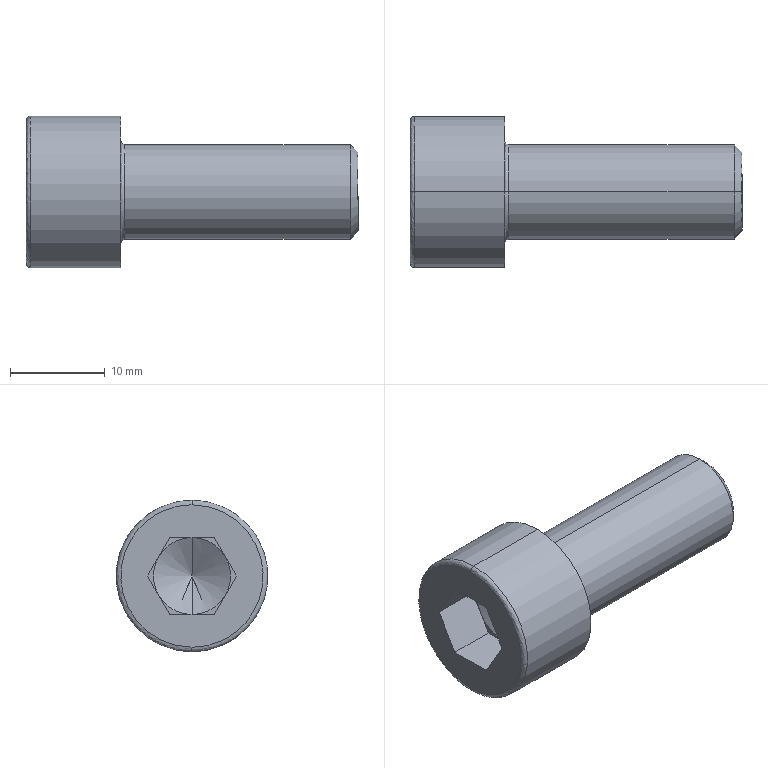Part | STEP file | PN_0009_default | 1 solid | 27 faces | box 35 x 16 x 16 mm | volume 3637 mm3 | plane 15 | spline 4 | cylinder 4 | cone 4 | commonest cylinder face diameters 10 x2 16 x2